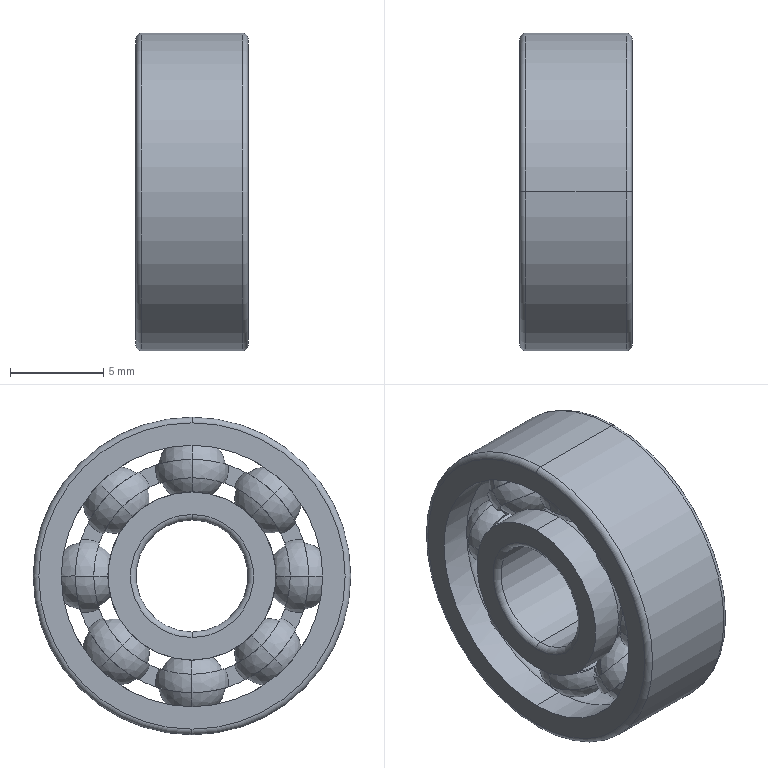Part | NX | features BREP 1 | 1 solid | 132 faces | box 6 x 17 x 17 mm | volume 795.711 mm3 | sphere 64 | torus 32 | plane 20 | cylinder 16 | commonest cylinder face diameters 9 x4 14 x4 6 x2 10.51 x2 12.49 x2 17 x2